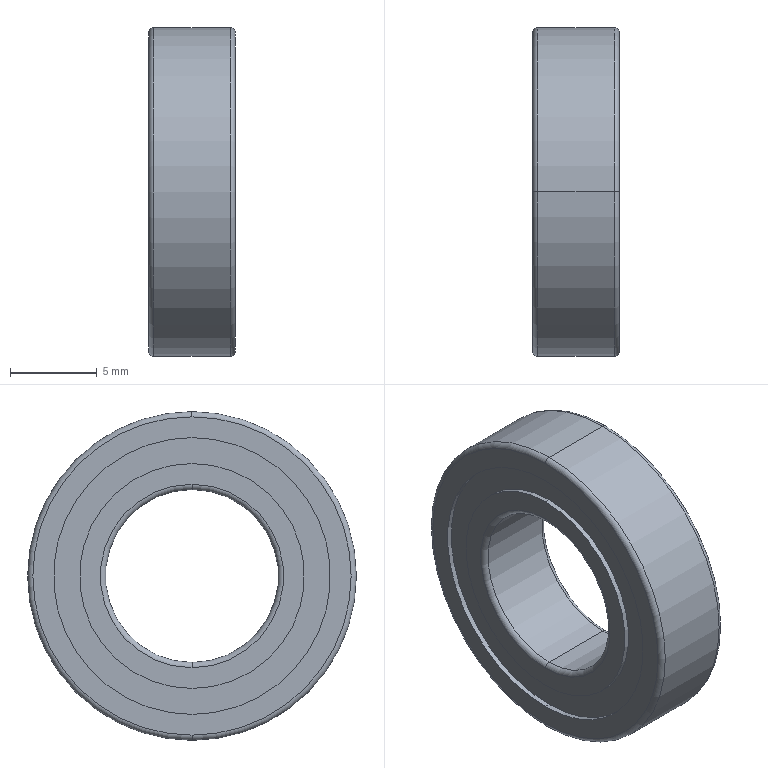Part | STEP file | 61800ZZ_Rolling bearings 61800 GB 276-94 | 1 solid | 134 faces | box 5 x 19 x 19 mm | volume 823.307 mm3 | torus 68 | sphere 38 | cylinder 20 | plane 8 | commonest cylinder face diameters 13 x8 16 x8 10 x2 19 x2